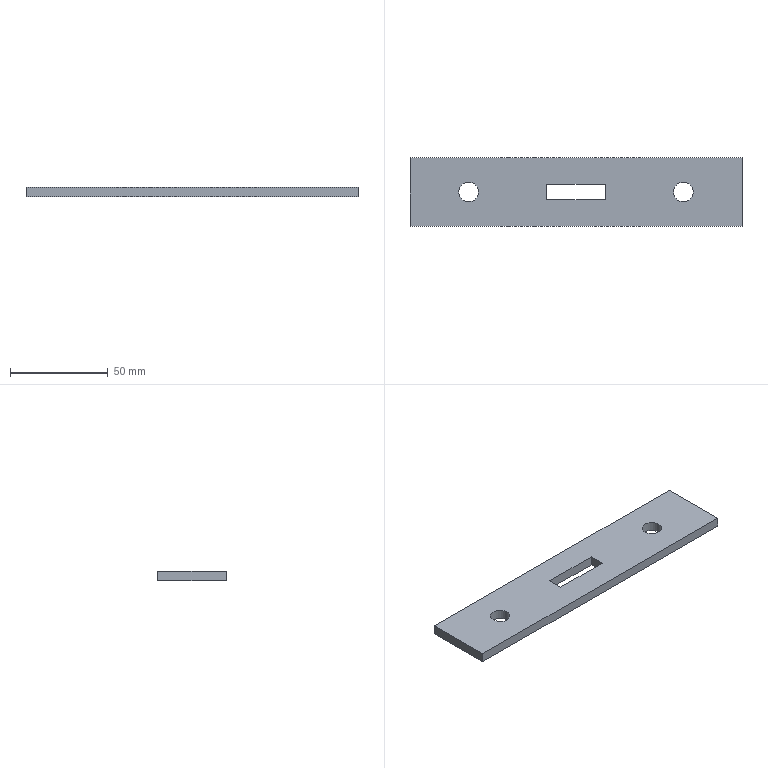Part | NX | features BREP 1 | 1 solid | 12 faces | box 170 x 35 x 5 mm | volume 27765 mm3 | plane 10 | cylinder 2 | commonest cylinder face diameters 10 x2
STEP:
#1=CARTESIAN_POINT('',(-60.,0.,5.));
#2=VERTEX_POINT('',#1);
#3=CARTESIAN_POINT('',(-55.,0.,5.));
#4=DIRECTION('',(0.,0.,1.));
#5=DIRECTION('',(-1.,0.,0.));
#6=AXIS2_PLACEMENT_3D('',#3,#4,#5);
#7=CIRCLE('',#6,5.);
#8=EDGE_CURVE('',#2,#2,#7,.T.);
#9=ORIENTED_EDGE('',*,*,#8,.T.);
#10=EDGE_LOOP('',(#9));
#11=FACE_BOUND('',#10,.T.);
#12=CARTESIAN_POINT('',(-50.,0.,0.));
#13=VERTEX_POINT('',#12);
#14=CARTESIAN_POINT('',(-55.,0.,0.));
#15=DIRECTION('',(0.,0.,1.));
#16=DIRECTION('',(1.,0.,0.));
#17=AXIS2_PLACEMENT_3D('',#14,#15,#16);
#18=CIRCLE('',#17,5.);
#19=EDGE_CURVE('',#13,#13,#18,.T.);
#20=ORIENTED_EDGE('',*,*,#19,.F.);
#21=EDGE_LOOP('',(#20));
#22=FACE_BOUND('',#21,.T.);
#23=CARTESIAN_POINT('',(-55.,0.,-10.));
#24=DIRECTION('',(0.,0.,1.));
#25=DIRECTION('',(1.,0.,0.));
#26=AXIS2_PLACEMENT_3D('',#23,#24,#25);
#27=CYLINDRICAL_SURFACE('',#26,5.);
#28=ADVANCED_FACE('',(#11,#22),#27,.F.);
#29=CARTESIAN_POINT('',(60.,0.,5.));
#30=VERTEX_POINT('',#29);
#31=CARTESIAN_POINT('',(55.,0.,5.));
#32=DIRECTION('',(0.,0.,1.));
#33=DIRECTION('',(1.,0.,0.));
#34=AXIS2_PLACEMENT_3D('',#31,#32,#33);
#35=CIRCLE('',#34,5.);
#36=EDGE_CURVE('',#30,#30,#35,.T.);
#37=ORIENTED_EDGE('',*,*,#36,.T.);
#38=EDGE_LOOP('',(#37));
#39=FACE_BOUND('',#38,.T.);
#40=CARTESIAN_POINT('',(60.,0.,0.));
#41=VERTEX_POINT('',#40);
#42=CARTESIAN_POINT('',(55.,0.,0.));
#43=DIRECTION('',(0.,0.,1.));
#44=DIRECTION('',(1.,0.,0.));
#45=AXIS2_PLACEMENT_3D('',#42,#43,#44);
#46=CIRCLE('',#45,5.);
#47=EDGE_CURVE('',#41,#41,#46,.T.);
#48=ORIENTED_EDGE('',*,*,#47,.F.);
#49=EDGE_LOOP('',(#48));
#50=FACE_BOUND('',#49,.T.);
#51=CARTESIAN_POINT('',(55.,0.,-10.));
#52=DIRECTION('',(0.,0.,1.));
#53=DIRECTION('',(1.,0.,0.));
#54=AXIS2_PLACEMENT_3D('',#51,#52,#53);
#55=CYLINDRICAL_SURFACE('',#54,5.);
#56=ADVANCED_FACE('',(#39,#50),#55,.F.);
#57=CARTESIAN_POINT('',(-85.,17.5,0.));
#58=VERTEX_POINT('',#57);
#59=CARTESIAN_POINT('',(-85.,-17.5,0.));
#60=VERTEX_POINT('',#59);
#61=CARTESIAN_POINT('',(-85.,-17.5,0.));
#62=DIRECTION('',(0.,-1.,0.));
#63=VECTOR('',#62,1000.);
#64=LINE('',#61,#63);
#65=EDGE_CURVE('',#58,#60,#64,.T.);
#66=ORIENTED_EDGE('',*,*,#65,.T.);
#67=CARTESIAN_POINT('',(-85.,-17.5,5.));
#68=VERTEX_POINT('',#67);
#69=CARTESIAN_POINT('',(-85.,-17.5,5.));
#70=DIRECTION('',(0.,0.,-1.));
#71=VECTOR('',#70,1000.);
#72=LINE('',#69,#71);
#73=EDGE_CURVE('',#68,#60,#72,.T.);
#74=ORIENTED_EDGE('',*,*,#73,.F.);
#75=CARTESIAN_POINT('',(-85.,17.5,5.));
#76=VERTEX_POINT('',#75);
#77=CARTESIAN_POINT('',(-85.,-17.5,5.));
#78=DIRECTION('',(0.,-1.,0.));
#79=VECTOR('',#78,1000.);
#80=LINE('',#77,#79);
#81=EDGE_CURVE('',#76,#68,#80,.T.);
#82=ORIENTED_EDGE('',*,*,#81,.F.);
#83=CARTESIAN_POINT('',(-85.,17.5,5.));
#84=DIRECTION('',(0.,0.,-1.));
#85=VECTOR('',#84,1000.);
#86=LINE('',#83,#85);
#87=EDGE_CURVE('',#76,#58,#86,.T.);
#88=ORIENTED_EDGE('',*,*,#87,.T.);
#89=EDGE_LOOP('',(#66,#74,#82,#88));
#90=FACE_BOUND('',#89,.T.);
#91=CARTESIAN_POINT('',(-85.,-17.5,5.));
#92=DIRECTION('',(1.,0.,0.));
#93=DIRECTION('',(0.,0.,-1.));
#94=AXIS2_PLACEMENT_3D('',#91,#92,#93);
#95=PLANE('',#94);
#96=ADVANCED_FACE('',(#90),#95,.F.);
#97=CARTESIAN_POINT('',(85.,-17.5,0.));
#98=VERTEX_POINT('',#97);
#99=CARTESIAN_POINT('',(-85.,-17.5,0.));
#100=DIRECTION('',(1.,0.,0.));
#101=VECTOR('',#100,1000.);
#102=LINE('',#99,#101);
#103=EDGE_CURVE('',#60,#98,#102,.T.);
#104=ORIENTED_EDGE('',*,*,#103,.T.);
#105=CARTESIAN_POINT('',(85.,-17.5,5.));
#106=VERTEX_POINT('',#105);
#107=CARTESIAN_POINT('',(85.,-17.5,5.));
#108=DIRECTION('',(0.,0.,-1.));
#109=VECTOR('',#108,1000.);
#110=LINE('',#107,#109);
#111=EDGE_CURVE('',#106,#98,#110,.T.);
#112=ORIENTED_EDGE('',*,*,#111,.F.);
#113=CARTESIAN_POINT('',(-85.,-17.5,5.));
#114=DIRECTION('',(1.,0.,0.));
#115=VECTOR('',#114,1000.);
#116=LINE('',#113,#115);
#117=EDGE_CURVE('',#68,#106,#116,.T.);
#118=ORIENTED_EDGE('',*,*,#117,.F.);
#119=ORIENTED_EDGE('',*,*,#73,.T.);
#120=EDGE_LOOP('',(#104,#112,#118,#119));
#121=FACE_BOUND('',#120,.T.);
#122=CARTESIAN_POINT('',(-85.,-17.5,5.));
#123=DIRECTION('',(0.,1.,0.));
#124=DIRECTION('',(0.,0.,1.));
#125=AXIS2_PLACEMENT_3D('',#122,#123,#124);
#126=PLANE('',#125);
#127=ADVANCED_FACE('',(#121),#126,.F.);
#128=CARTESIAN_POINT('',(85.,17.5,0.));
#129=VERTEX_POINT('',#128);
#130=CARTESIAN_POINT('',(85.,-17.5,0.));
#131=DIRECTION('',(0.,1.,0.));
#132=VECTOR('',#131,1000.);
#133=LINE('',#130,#132);
#134=EDGE_CURVE('',#98,#129,#133,.T.);
#135=ORIENTED_EDGE('',*,*,#134,.T.);
#136=CARTESIAN_POINT('',(85.,17.5,5.));
#137=VERTEX_POINT('',#136);
#138=CARTESIAN_POINT('',(85.,17.5,5.));
#139=DIRECTION('',(0.,0.,-1.));
#140=VECTOR('',#139,1000.);
#141=LINE('',#138,#140);
#142=EDGE_CURVE('',#137,#129,#141,.T.);
#143=ORIENTED_EDGE('',*,*,#142,.F.);
#144=CARTESIAN_POINT('',(85.,-17.5,5.));
#145=DIRECTION('',(0.,1.,0.));
#146=VECTOR('',#145,1000.);
#147=LINE('',#144,#146);
#148=EDGE_CURVE('',#106,#137,#147,.T.);
#149=ORIENTED_EDGE('',*,*,#148,.F.);
#150=ORIENTED_EDGE('',*,*,#111,.T.);
#151=EDGE_LOOP('',(#135,#143,#149,#150));
#152=FACE_BOUND('',#151,.T.);
#153=CARTESIAN_POINT('',(85.,-17.5,5.));
#154=DIRECTION('',(-1.,0.,0.));
#155=DIRECTION('',(0.,0.,1.));
#156=AXIS2_PLACEMENT_3D('',#153,#154,#155);
#157=PLANE('',#156);
#158=ADVANCED_FACE('',(#152),#157,.F.);
#159=CARTESIAN_POINT('',(85.,17.5,0.));
#160=DIRECTION('',(-1.,0.,0.));
#161=VECTOR('',#160,1000.);
#162=LINE('',#159,#161);
#163=EDGE_CURVE('',#129,#58,#162,.T.);
#164=ORIENTED_EDGE('',*,*,#163,.T.);
#165=ORIENTED_EDGE('',*,*,#87,.F.);
#166=CARTESIAN_POINT('',(85.,17.5,5.));
#167=DIRECTION('',(-1.,0.,0.));
#168=VECTOR('',#167,1000.);
#169=LINE('',#166,#168);
#170=EDGE_CURVE('',#137,#76,#169,.T.);
#171=ORIENTED_EDGE('',*,*,#170,.F.);
#172=ORIENTED_EDGE('',*,*,#142,.T.);
#173=EDGE_LOOP('',(#164,#165,#171,#172));
#174=FACE_BOUND('',#173,.T.);
#175=CARTESIAN_POINT('',(85.,17.5,5.));
#176=DIRECTION('',(0.,-1.,0.));
#177=DIRECTION('',(1.,0.,0.));
#178=AXIS2_PLACEMENT_3D('',#175,#176,#177);
#179=PLANE('',#178);
#180=ADVANCED_FACE('',(#174),#179,.F.);
#181=CARTESIAN_POINT('',(-15.,4.,5.));
#182=VERTEX_POINT('',#181);
#183=CARTESIAN_POINT('',(-15.,-4.,5.));
#184=VERTEX_POINT('',#183);
#185=CARTESIAN_POINT('',(-15.,-4.,5.));
#186=DIRECTION('',(0.,-1.,0.));
#187=VECTOR('',#186,1000.);
#188=LINE('',#185,#187);
#189=EDGE_CURVE('',#182,#184,#188,.T.);
#190=ORIENTED_EDGE('',*,*,#189,.F.);
#191=CARTESIAN_POINT('',(15.,4.,5.));
#192=VERTEX_POINT('',#191);
#193=CARTESIAN_POINT('',(-15.,4.,5.));
#194=DIRECTION('',(-1.,0.,0.));
#195=VECTOR('',#194,1000.);
#196=LINE('',#193,#195);
#197=EDGE_CURVE('',#192,#182,#196,.T.);
#198=ORIENTED_EDGE('',*,*,#197,.F.);
#199=CARTESIAN_POINT('',(15.,-4.,5.));
#200=VERTEX_POINT('',#199);
#201=CARTESIAN_POINT('',(15.,-4.,5.));
#202=DIRECTION('',(0.,1.,0.));
#203=VECTOR('',#202,1000.);
#204=LINE('',#201,#203);
#205=EDGE_CURVE('',#200,#192,#204,.T.);
#206=ORIENTED_EDGE('',*,*,#205,.F.);
#207=CARTESIAN_POINT('',(-15.,-4.,5.));
#208=DIRECTION('',(1.,0.,0.));
#209=VECTOR('',#208,1000.);
#210=LINE('',#207,#209);
#211=EDGE_CURVE('',#184,#200,#210,.T.);
#212=ORIENTED_EDGE('',*,*,#211,.F.);
#213=EDGE_LOOP('',(#190,#198,#206,#212));
#214=FACE_BOUND('',#213,.T.);
#215=ORIENTED_EDGE('',*,*,#8,.F.);
#216=EDGE_LOOP('',(#215));
#217=FACE_BOUND('',#216,.T.);
#218=ORIENTED_EDGE('',*,*,#36,.F.);
#219=EDGE_LOOP('',(#218));
#220=FACE_BOUND('',#219,.T.);
#221=ORIENTED_EDGE('',*,*,#81,.T.);
#222=ORIENTED_EDGE('',*,*,#117,.T.);
#223=ORIENTED_EDGE('',*,*,#148,.T.);
#224=ORIENTED_EDGE('',*,*,#170,.T.);
#225=EDGE_LOOP('',(#221,#222,#223,#224));
#226=FACE_BOUND('',#225,.T.);
#227=CARTESIAN_POINT('',(0.,0.,5.));
#228=DIRECTION('',(0.,0.,1.));
#229=DIRECTION('',(1.,0.,0.));
#230=AXIS2_PLACEMENT_3D('',#227,#228,#229);
#231=PLANE('',#230);
#232=ADVANCED_FACE('',(#214,#217,#220,#226),#231,.T.);
#233=CARTESIAN_POINT('',(15.,4.,0.));
#234=VERTEX_POINT('',#233);
#235=CARTESIAN_POINT('',(-15.,4.,0.));
#236=VERTEX_POINT('',#235);
#237=CARTESIAN_POINT('',(0.,4.,0.));
#238=DIRECTION('',(-1.,0.,0.));
#239=VECTOR('',#238,1000.);
#240=LINE('',#237,#239);
#241=EDGE_CURVE('',#234,#236,#240,.T.);
#242=ORIENTED_EDGE('',*,*,#241,.T.);
#243=CARTESIAN_POINT('',(-15.,-4.,0.));
#244=VERTEX_POINT('',#243);
#245=CARTESIAN_POINT('',(-15.,0.,0.));
#246=DIRECTION('',(0.,-1.,0.));
#247=VECTOR('',#246,1000.);
#248=LINE('',#245,#247);
#249=EDGE_CURVE('',#236,#244,#248,.T.);
#250=ORIENTED_EDGE('',*,*,#249,.T.);
#251=CARTESIAN_POINT('',(15.,-4.,0.));
#252=VERTEX_POINT('',#251);
#253=CARTESIAN_POINT('',(0.,-4.,0.));
#254=DIRECTION('',(1.,0.,0.));
#255=VECTOR('',#254,1000.);
#256=LINE('',#253,#255);
#257=EDGE_CURVE('',#244,#252,#256,.T.);
#258=ORIENTED_EDGE('',*,*,#257,.T.);
#259=CARTESIAN_POINT('',(15.,0.,0.));
#260=DIRECTION('',(0.,1.,0.));
#261=VECTOR('',#260,1000.);
#262=LINE('',#259,#261);
#263=EDGE_CURVE('',#252,#234,#262,.T.);
#264=ORIENTED_EDGE('',*,*,#263,.T.);
#265=EDGE_LOOP('',(#242,#250,#258,#264));
#266=FACE_BOUND('',#265,.T.);
#267=ORIENTED_EDGE('',*,*,#19,.T.);
#268=EDGE_LOOP('',(#267));
#269=FACE_BOUND('',#268,.T.);
#270=ORIENTED_EDGE('',*,*,#47,.T.);
#271=EDGE_LOOP('',(#270));
#272=FACE_BOUND('',#271,.T.);
#273=ORIENTED_EDGE('',*,*,#65,.F.);
#274=ORIENTED_EDGE('',*,*,#163,.F.);
#275=ORIENTED_EDGE('',*,*,#134,.F.);
#276=ORIENTED_EDGE('',*,*,#103,.F.);
#277=EDGE_LOOP('',(#273,#274,#275,#276));
#278=FACE_BOUND('',#277,.T.);
#279=CARTESIAN_POINT('',(0.,0.,0.));
#280=DIRECTION('',(0.,0.,1.));
#281=DIRECTION('',(1.,0.,0.));
#282=AXIS2_PLACEMENT_3D('',#279,#280,#281);
#283=PLANE('',#282);
#284=ADVANCED_FACE('',(#266,#269,#272,#278),#283,.F.);
#285=CARTESIAN_POINT('',(-15.,4.,-10.));
#286=DIRECTION('',(0.,0.,1.));
#287=VECTOR('',#286,1000.);
#288=LINE('',#285,#287);
#289=EDGE_CURVE('',#236,#182,#288,.T.);
#290=ORIENTED_EDGE('',*,*,#289,.T.);
#291=ORIENTED_EDGE('',*,*,#189,.T.);
#292=CARTESIAN_POINT('',(-15.,-4.,-10.));
#293=DIRECTION('',(0.,0.,1.));
#294=VECTOR('',#293,1000.);
#295=LINE('',#292,#294);
#296=EDGE_CURVE('',#244,#184,#295,.T.);
#297=ORIENTED_EDGE('',*,*,#296,.F.);
#298=ORIENTED_EDGE('',*,*,#249,.F.);
#299=EDGE_LOOP('',(#290,#291,#297,#298));
#300=FACE_BOUND('',#299,.T.);
#301=CARTESIAN_POINT('',(-15.,-4.,-10.));
#302=DIRECTION('',(-1.,0.,0.));
#303=DIRECTION('',(0.,0.,1.));
#304=AXIS2_PLACEMENT_3D('',#301,#302,#303);
#305=PLANE('',#304);
#306=ADVANCED_FACE('',(#300),#305,.F.);
#307=CARTESIAN_POINT('',(15.,4.,-10.));
#308=DIRECTION('',(0.,0.,1.));
#309=VECTOR('',#308,1000.);
#310=LINE('',#307,#309);
#311=EDGE_CURVE('',#234,#192,#310,.T.);
#312=ORIENTED_EDGE('',*,*,#311,.T.);
#313=ORIENTED_EDGE('',*,*,#197,.T.);
#314=ORIENTED_EDGE('',*,*,#289,.F.);
#315=ORIENTED_EDGE('',*,*,#241,.F.);
#316=EDGE_LOOP('',(#312,#313,#314,#315));
#317=FACE_BOUND('',#316,.T.);
#318=CARTESIAN_POINT('',(-15.,4.,-10.));
#319=DIRECTION('',(0.,1.,0.));
#320=DIRECTION('',(-1.,0.,0.));
#321=AXIS2_PLACEMENT_3D('',#318,#319,#320);
#322=PLANE('',#321);
#323=ADVANCED_FACE('',(#317),#322,.F.);
#324=CARTESIAN_POINT('',(15.,-4.,-10.));
#325=DIRECTION('',(0.,0.,1.));
#326=VECTOR('',#325,1000.);
#327=LINE('',#324,#326);
#328=EDGE_CURVE('',#252,#200,#327,.T.);
#329=ORIENTED_EDGE('',*,*,#328,.T.);
#330=ORIENTED_EDGE('',*,*,#205,.T.);
#331=ORIENTED_EDGE('',*,*,#311,.F.);
#332=ORIENTED_EDGE('',*,*,#263,.F.);
#333=EDGE_LOOP('',(#329,#330,#331,#332));
#334=FACE_BOUND('',#333,.T.);
#335=CARTESIAN_POINT('',(15.,-4.,-10.));
#336=DIRECTION('',(1.,0.,0.));
#337=DIRECTION('',(0.,1.,0.));
#338=AXIS2_PLACEMENT_3D('',#335,#336,#337);
#339=PLANE('',#338);
#340=ADVANCED_FACE('',(#334),#339,.F.);
#341=ORIENTED_EDGE('',*,*,#296,.T.);
#342=ORIENTED_EDGE('',*,*,#211,.T.);
#343=ORIENTED_EDGE('',*,*,#328,.F.);
#344=ORIENTED_EDGE('',*,*,#257,.F.);
#345=EDGE_LOOP('',(#341,#342,#343,#344));
#346=FACE_BOUND('',#345,.T.);
#347=CARTESIAN_POINT('',(-15.,-4.,-10.));
#348=DIRECTION('',(0.,-1.,0.));
#349=DIRECTION('',(1.,0.,0.));
#350=AXIS2_PLACEMENT_3D('',#347,#348,#349);
#351=PLANE('',#350);
#352=ADVANCED_FACE('',(#346),#351,.F.);
#353=CLOSED_SHELL('',(#28,#56,#96,#127,#158,#180,#232,#284,#306,#323,#340,#352));
#354=MANIFOLD_SOLID_BREP('',#353);
#355=(LENGTH_UNIT()NAMED_UNIT(*)SI_UNIT(.MILLI.,.METRE.));
#356=UNCERTAINTY_MEASURE_WITH_UNIT(LENGTH_MEASURE(0.00001),#355,'','');
#357=(NAMED_UNIT(*)PLANE_ANGLE_UNIT()SI_UNIT($,.RADIAN.));
#358=(NAMED_UNIT(*)SI_UNIT($,.STERADIAN.)SOLID_ANGLE_UNIT());
#359=(GEOMETRIC_REPRESENTATION_CONTEXT(3)GLOBAL_UNCERTAINTY_ASSIGNED_CONTEXT((#356))GLOBAL_UNIT_ASSIGNED_CONTEXT((#355,#357,#358))REPRESENTATION_CONTEXT('',''));
#360=ADVANCED_BREP_SHAPE_REPRESENTATION('',(#354),#359);